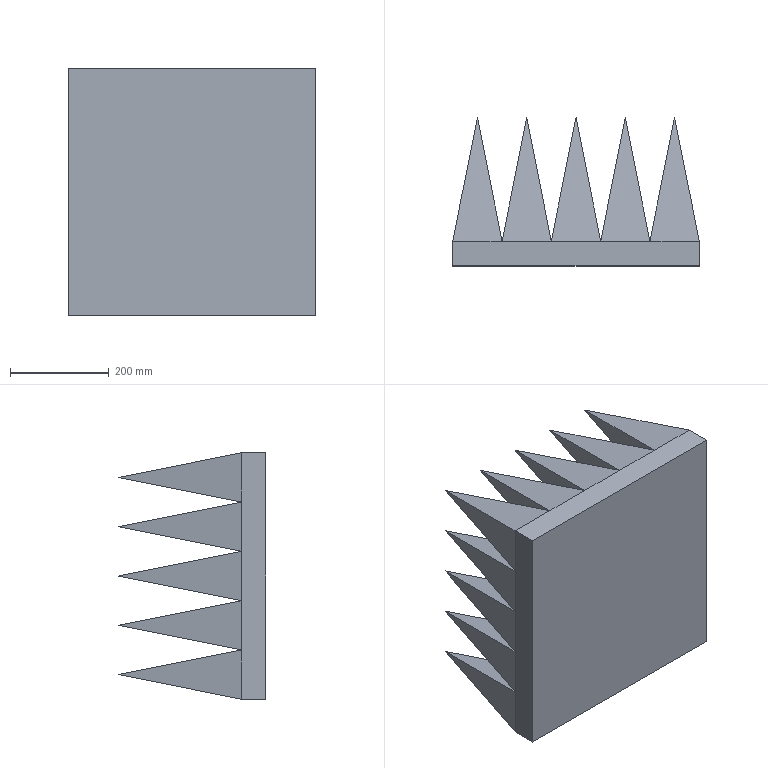Part | SolidWorks | features LPattern 2, Blend 1, Extrusion 1, ICE 1 | 1 solid | 105 faces | box 500 x 300 x 500 mm | volume 33333333 mm3 | plane 105